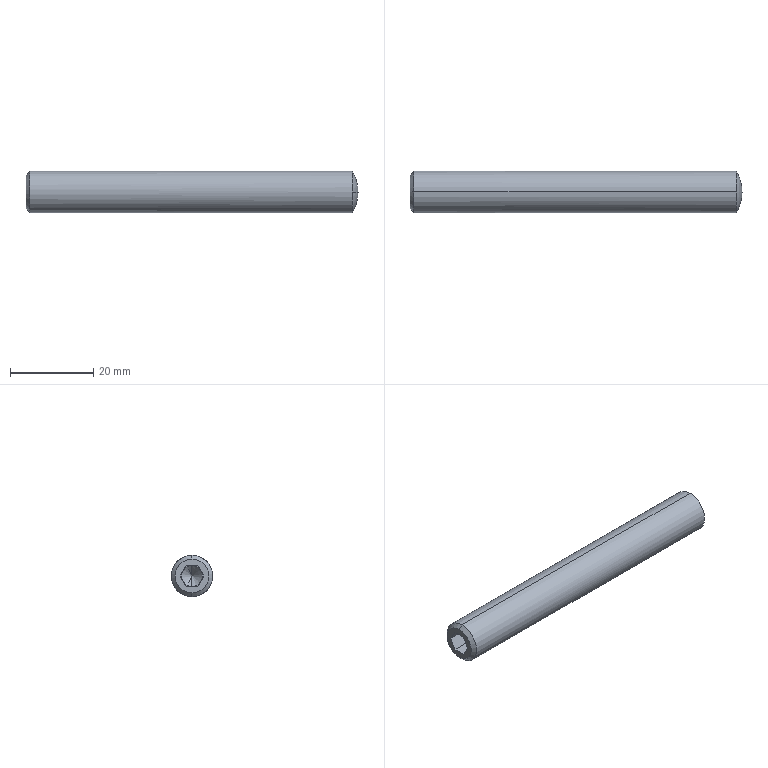Part | STEP file | 0217_Z_ANBNS10-80-1 | 1 solid | 21 faces | box 80 x 10 x 10 mm | volume 6095 mm3 | plane 13 | cone 4 | spline 2 | cylinder 2 | commonest cylinder face diameters 10 x2